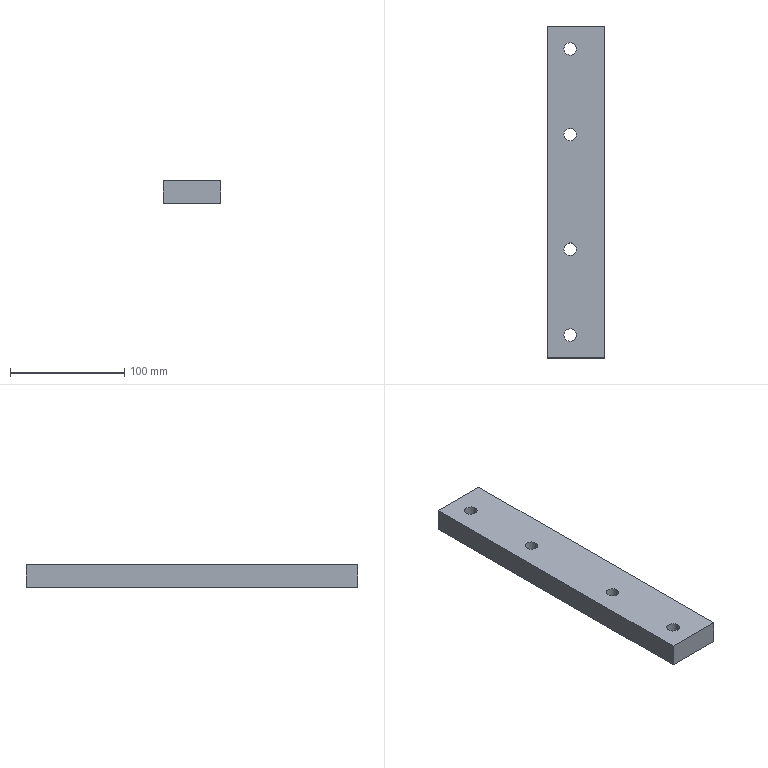Part | SolidWorks | features Extrusion 1, HoleWzd 1 | 1 solid | 14 faces | box 50 x 290 x 20 mm | volume 282397 mm3 | cylinder 8 | plane 6 | commonest cylinder face diameters 11 x8
STEP:
#1=CARTESIAN_POINT('',(0.5,125.,0.));
#2=VERTEX_POINT('',#1);
#3=CARTESIAN_POINT('',(-10.5,125.,0.));
#4=VERTEX_POINT('',#3);
#5=CARTESIAN_POINT('',(-5.,125.,0.));
#6=DIRECTION('',(0.,0.,-1.));
#7=DIRECTION('',(-1.,0.,0.));
#8=AXIS2_PLACEMENT_3D('',#5,#6,#7);
#9=CIRCLE('',#8,5.5);
#10=EDGE_CURVE('',#2,#4,#9,.T.);
#11=ORIENTED_EDGE('',*,*,#10,.T.);
#12=CARTESIAN_POINT('',(-10.5,125.,20.));
#13=VERTEX_POINT('',#12);
#14=CARTESIAN_POINT('',(-10.5,125.,20.));
#15=DIRECTION('',(0.,0.,1.));
#16=VECTOR('',#15,1000.);
#17=LINE('',#14,#16);
#18=EDGE_CURVE('',#4,#13,#17,.T.);
#19=ORIENTED_EDGE('',*,*,#18,.T.);
#20=CARTESIAN_POINT('',(0.5,125.,20.));
#21=VERTEX_POINT('',#20);
#22=CARTESIAN_POINT('',(-5.,125.,20.));
#23=DIRECTION('',(0.,0.,1.));
#24=DIRECTION('',(1.,0.,0.));
#25=AXIS2_PLACEMENT_3D('',#22,#23,#24);
#26=CIRCLE('',#25,5.5);
#27=EDGE_CURVE('',#13,#21,#26,.T.);
#28=ORIENTED_EDGE('',*,*,#27,.T.);
#29=CARTESIAN_POINT('',(0.5,125.,20.));
#30=DIRECTION('',(0.,0.,1.));
#31=VECTOR('',#30,1000.);
#32=LINE('',#29,#31);
#33=EDGE_CURVE('',#2,#21,#32,.T.);
#34=ORIENTED_EDGE('',*,*,#33,.F.);
#35=EDGE_LOOP('',(#11,#19,#28,#34));
#36=FACE_OUTER_BOUND('',#35,.T.);
#37=CARTESIAN_POINT('',(-5.,125.,20.));
#38=DIRECTION('',(0.,0.,1.));
#39=DIRECTION('',(1.,0.,0.));
#40=AXIS2_PLACEMENT_3D('',#37,#38,#39);
#41=CYLINDRICAL_SURFACE('',#40,5.5);
#42=ADVANCED_FACE('',(#36),#41,.F.);
#43=CARTESIAN_POINT('',(0.5,50.,0.));
#44=VERTEX_POINT('',#43);
#45=CARTESIAN_POINT('',(-10.5,50.,0.));
#46=VERTEX_POINT('',#45);
#47=CARTESIAN_POINT('',(-5.,50.,0.));
#48=DIRECTION('',(0.,0.,-1.));
#49=DIRECTION('',(-1.,0.,0.));
#50=AXIS2_PLACEMENT_3D('',#47,#48,#49);
#51=CIRCLE('',#50,5.5);
#52=EDGE_CURVE('',#44,#46,#51,.T.);
#53=ORIENTED_EDGE('',*,*,#52,.T.);
#54=CARTESIAN_POINT('',(-10.5,50.,20.));
#55=VERTEX_POINT('',#54);
#56=CARTESIAN_POINT('',(-10.5,50.,20.));
#57=DIRECTION('',(0.,0.,1.));
#58=VECTOR('',#57,1000.);
#59=LINE('',#56,#58);
#60=EDGE_CURVE('',#46,#55,#59,.T.);
#61=ORIENTED_EDGE('',*,*,#60,.T.);
#62=CARTESIAN_POINT('',(0.5,50.,20.));
#63=VERTEX_POINT('',#62);
#64=CARTESIAN_POINT('',(-5.,50.,20.));
#65=DIRECTION('',(0.,0.,1.));
#66=DIRECTION('',(1.,0.,0.));
#67=AXIS2_PLACEMENT_3D('',#64,#65,#66);
#68=CIRCLE('',#67,5.5);
#69=EDGE_CURVE('',#55,#63,#68,.T.);
#70=ORIENTED_EDGE('',*,*,#69,.T.);
#71=CARTESIAN_POINT('',(0.5,50.,20.));
#72=DIRECTION('',(0.,0.,1.));
#73=VECTOR('',#72,1000.);
#74=LINE('',#71,#73);
#75=EDGE_CURVE('',#44,#63,#74,.T.);
#76=ORIENTED_EDGE('',*,*,#75,.F.);
#77=EDGE_LOOP('',(#53,#61,#70,#76));
#78=FACE_OUTER_BOUND('',#77,.T.);
#79=CARTESIAN_POINT('',(-5.,50.,20.));
#80=DIRECTION('',(0.,0.,1.));
#81=DIRECTION('',(1.,0.,0.));
#82=AXIS2_PLACEMENT_3D('',#79,#80,#81);
#83=CYLINDRICAL_SURFACE('',#82,5.5);
#84=ADVANCED_FACE('',(#78),#83,.F.);
#85=CARTESIAN_POINT('',(0.5,-50.,0.));
#86=VERTEX_POINT('',#85);
#87=CARTESIAN_POINT('',(-10.5,-50.,0.));
#88=VERTEX_POINT('',#87);
#89=CARTESIAN_POINT('',(-5.,-50.,0.));
#90=DIRECTION('',(0.,0.,-1.));
#91=DIRECTION('',(-1.,0.,0.));
#92=AXIS2_PLACEMENT_3D('',#89,#90,#91);
#93=CIRCLE('',#92,5.5);
#94=EDGE_CURVE('',#86,#88,#93,.T.);
#95=ORIENTED_EDGE('',*,*,#94,.T.);
#96=CARTESIAN_POINT('',(-10.5,-50.,20.));
#97=VERTEX_POINT('',#96);
#98=CARTESIAN_POINT('',(-10.5,-50.,20.));
#99=DIRECTION('',(0.,0.,1.));
#100=VECTOR('',#99,1000.);
#101=LINE('',#98,#100);
#102=EDGE_CURVE('',#88,#97,#101,.T.);
#103=ORIENTED_EDGE('',*,*,#102,.T.);
#104=CARTESIAN_POINT('',(0.5,-50.,20.));
#105=VERTEX_POINT('',#104);
#106=CARTESIAN_POINT('',(-5.,-50.,20.));
#107=DIRECTION('',(0.,0.,1.));
#108=DIRECTION('',(1.,0.,0.));
#109=AXIS2_PLACEMENT_3D('',#106,#107,#108);
#110=CIRCLE('',#109,5.5);
#111=EDGE_CURVE('',#97,#105,#110,.T.);
#112=ORIENTED_EDGE('',*,*,#111,.T.);
#113=CARTESIAN_POINT('',(0.5,-50.,20.));
#114=DIRECTION('',(0.,0.,1.));
#115=VECTOR('',#114,1000.);
#116=LINE('',#113,#115);
#117=EDGE_CURVE('',#86,#105,#116,.T.);
#118=ORIENTED_EDGE('',*,*,#117,.F.);
#119=EDGE_LOOP('',(#95,#103,#112,#118));
#120=FACE_OUTER_BOUND('',#119,.T.);
#121=CARTESIAN_POINT('',(-5.,-50.,20.));
#122=DIRECTION('',(0.,0.,1.));
#123=DIRECTION('',(1.,0.,0.));
#124=AXIS2_PLACEMENT_3D('',#121,#122,#123);
#125=CYLINDRICAL_SURFACE('',#124,5.5);
#126=ADVANCED_FACE('',(#120),#125,.F.);
#127=CARTESIAN_POINT('',(0.5,-125.,0.));
#128=VERTEX_POINT('',#127);
#129=CARTESIAN_POINT('',(-10.5,-125.,0.));
#130=VERTEX_POINT('',#129);
#131=CARTESIAN_POINT('',(-5.,-125.,0.));
#132=DIRECTION('',(0.,0.,-1.));
#133=DIRECTION('',(-1.,0.,0.));
#134=AXIS2_PLACEMENT_3D('',#131,#132,#133);
#135=CIRCLE('',#134,5.5);
#136=EDGE_CURVE('',#128,#130,#135,.T.);
#137=ORIENTED_EDGE('',*,*,#136,.T.);
#138=CARTESIAN_POINT('',(-10.5,-125.,20.));
#139=VERTEX_POINT('',#138);
#140=CARTESIAN_POINT('',(-10.5,-125.,20.));
#141=DIRECTION('',(0.,0.,1.));
#142=VECTOR('',#141,1000.);
#143=LINE('',#140,#142);
#144=EDGE_CURVE('',#130,#139,#143,.T.);
#145=ORIENTED_EDGE('',*,*,#144,.T.);
#146=CARTESIAN_POINT('',(0.5,-125.,20.));
#147=VERTEX_POINT('',#146);
#148=CARTESIAN_POINT('',(-5.,-125.,20.));
#149=DIRECTION('',(0.,0.,1.));
#150=DIRECTION('',(1.,0.,0.));
#151=AXIS2_PLACEMENT_3D('',#148,#149,#150);
#152=CIRCLE('',#151,5.5);
#153=EDGE_CURVE('',#139,#147,#152,.T.);
#154=ORIENTED_EDGE('',*,*,#153,.T.);
#155=CARTESIAN_POINT('',(0.5,-125.,20.));
#156=DIRECTION('',(0.,0.,1.));
#157=VECTOR('',#156,1000.);
#158=LINE('',#155,#157);
#159=EDGE_CURVE('',#128,#147,#158,.T.);
#160=ORIENTED_EDGE('',*,*,#159,.F.);
#161=EDGE_LOOP('',(#137,#145,#154,#160));
#162=FACE_OUTER_BOUND('',#161,.T.);
#163=CARTESIAN_POINT('',(-5.,-125.,20.));
#164=DIRECTION('',(0.,0.,1.));
#165=DIRECTION('',(1.,0.,0.));
#166=AXIS2_PLACEMENT_3D('',#163,#164,#165);
#167=CYLINDRICAL_SURFACE('',#166,5.5);
#168=ADVANCED_FACE('',(#162),#167,.F.);
#169=CARTESIAN_POINT('',(25.,-145.,0.));
#170=VERTEX_POINT('',#169);
#171=CARTESIAN_POINT('',(25.,145.,0.));
#172=VERTEX_POINT('',#171);
#173=CARTESIAN_POINT('',(25.,-145.,0.));
#174=DIRECTION('',(0.,1.,0.));
#175=VECTOR('',#174,1000.);
#176=LINE('',#173,#175);
#177=EDGE_CURVE('',#170,#172,#176,.T.);
#178=ORIENTED_EDGE('',*,*,#177,.T.);
#179=CARTESIAN_POINT('',(25.,145.,20.));
#180=VERTEX_POINT('',#179);
#181=CARTESIAN_POINT('',(25.,145.,20.));
#182=DIRECTION('',(0.,0.,-1.));
#183=VECTOR('',#182,1000.);
#184=LINE('',#181,#183);
#185=EDGE_CURVE('',#180,#172,#184,.T.);
#186=ORIENTED_EDGE('',*,*,#185,.F.);
#187=CARTESIAN_POINT('',(25.,-145.,20.));
#188=VERTEX_POINT('',#187);
#189=CARTESIAN_POINT('',(25.,-145.,20.));
#190=DIRECTION('',(0.,1.,0.));
#191=VECTOR('',#190,1000.);
#192=LINE('',#189,#191);
#193=EDGE_CURVE('',#188,#180,#192,.T.);
#194=ORIENTED_EDGE('',*,*,#193,.F.);
#195=CARTESIAN_POINT('',(25.,-145.,20.));
#196=DIRECTION('',(0.,0.,-1.));
#197=VECTOR('',#196,1000.);
#198=LINE('',#195,#197);
#199=EDGE_CURVE('',#188,#170,#198,.T.);
#200=ORIENTED_EDGE('',*,*,#199,.T.);
#201=EDGE_LOOP('',(#178,#186,#194,#200));
#202=FACE_OUTER_BOUND('',#201,.T.);
#203=CARTESIAN_POINT('',(25.,-145.,20.));
#204=DIRECTION('',(-1.,0.,0.));
#205=DIRECTION('',(0.,0.,1.));
#206=AXIS2_PLACEMENT_3D('',#203,#204,#205);
#207=PLANE('',#206);
#208=ADVANCED_FACE('',(#202),#207,.F.);
#209=CARTESIAN_POINT('',(-25.,145.,0.));
#210=VERTEX_POINT('',#209);
#211=CARTESIAN_POINT('',(-25.,145.,0.));
#212=DIRECTION('',(-1.,0.,0.));
#213=VECTOR('',#212,1000.);
#214=LINE('',#211,#213);
#215=EDGE_CURVE('',#172,#210,#214,.T.);
#216=ORIENTED_EDGE('',*,*,#215,.T.);
#217=CARTESIAN_POINT('',(-25.,145.,20.));
#218=VERTEX_POINT('',#217);
#219=CARTESIAN_POINT('',(-25.,145.,20.));
#220=DIRECTION('',(0.,0.,-1.));
#221=VECTOR('',#220,1000.);
#222=LINE('',#219,#221);
#223=EDGE_CURVE('',#218,#210,#222,.T.);
#224=ORIENTED_EDGE('',*,*,#223,.F.);
#225=CARTESIAN_POINT('',(-25.,145.,20.));
#226=DIRECTION('',(-1.,0.,0.));
#227=VECTOR('',#226,1000.);
#228=LINE('',#225,#227);
#229=EDGE_CURVE('',#180,#218,#228,.T.);
#230=ORIENTED_EDGE('',*,*,#229,.F.);
#231=ORIENTED_EDGE('',*,*,#185,.T.);
#232=EDGE_LOOP('',(#216,#224,#230,#231));
#233=FACE_OUTER_BOUND('',#232,.T.);
#234=CARTESIAN_POINT('',(-25.,145.,20.));
#235=DIRECTION('',(0.,-1.,0.));
#236=DIRECTION('',(0.,0.,-1.));
#237=AXIS2_PLACEMENT_3D('',#234,#235,#236);
#238=PLANE('',#237);
#239=ADVANCED_FACE('',(#233),#238,.F.);
#240=CARTESIAN_POINT('',(-25.,-145.,0.));
#241=VERTEX_POINT('',#240);
#242=CARTESIAN_POINT('',(-25.,-145.,0.));
#243=DIRECTION('',(0.,-1.,0.));
#244=VECTOR('',#243,1000.);
#245=LINE('',#242,#244);
#246=EDGE_CURVE('',#210,#241,#245,.T.);
#247=ORIENTED_EDGE('',*,*,#246,.T.);
#248=CARTESIAN_POINT('',(-25.,-145.,20.));
#249=VERTEX_POINT('',#248);
#250=CARTESIAN_POINT('',(-25.,-145.,20.));
#251=DIRECTION('',(0.,0.,-1.));
#252=VECTOR('',#251,1000.);
#253=LINE('',#250,#252);
#254=EDGE_CURVE('',#249,#241,#253,.T.);
#255=ORIENTED_EDGE('',*,*,#254,.F.);
#256=CARTESIAN_POINT('',(-25.,-145.,20.));
#257=DIRECTION('',(0.,-1.,0.));
#258=VECTOR('',#257,1000.);
#259=LINE('',#256,#258);
#260=EDGE_CURVE('',#218,#249,#259,.T.);
#261=ORIENTED_EDGE('',*,*,#260,.F.);
#262=ORIENTED_EDGE('',*,*,#223,.T.);
#263=EDGE_LOOP('',(#247,#255,#261,#262));
#264=FACE_OUTER_BOUND('',#263,.T.);
#265=CARTESIAN_POINT('',(-25.,-145.,20.));
#266=DIRECTION('',(1.,0.,0.));
#267=DIRECTION('',(0.,0.,-1.));
#268=AXIS2_PLACEMENT_3D('',#265,#266,#267);
#269=PLANE('',#268);
#270=ADVANCED_FACE('',(#264),#269,.F.);
#271=CARTESIAN_POINT('',(-25.,-145.,0.));
#272=DIRECTION('',(1.,0.,0.));
#273=VECTOR('',#272,1000.);
#274=LINE('',#271,#273);
#275=EDGE_CURVE('',#241,#170,#274,.T.);
#276=ORIENTED_EDGE('',*,*,#275,.T.);
#277=ORIENTED_EDGE('',*,*,#199,.F.);
#278=CARTESIAN_POINT('',(-25.,-145.,20.));
#279=DIRECTION('',(1.,0.,0.));
#280=VECTOR('',#279,1000.);
#281=LINE('',#278,#280);
#282=EDGE_CURVE('',#249,#188,#281,.T.);
#283=ORIENTED_EDGE('',*,*,#282,.F.);
#284=ORIENTED_EDGE('',*,*,#254,.T.);
#285=EDGE_LOOP('',(#276,#277,#283,#284));
#286=FACE_OUTER_BOUND('',#285,.T.);
#287=CARTESIAN_POINT('',(-25.,-145.,20.));
#288=DIRECTION('',(0.,1.,0.));
#289=DIRECTION('',(0.,0.,1.));
#290=AXIS2_PLACEMENT_3D('',#287,#288,#289);
#291=PLANE('',#290);
#292=ADVANCED_FACE('',(#286),#291,.F.);
#293=CARTESIAN_POINT('',(-5.,125.,20.));
#294=DIRECTION('',(0.,0.,1.));
#295=DIRECTION('',(1.,0.,0.));
#296=AXIS2_PLACEMENT_3D('',#293,#294,#295);
#297=CIRCLE('',#296,5.5);
#298=EDGE_CURVE('',#21,#13,#297,.T.);
#299=ORIENTED_EDGE('',*,*,#298,.F.);
#300=ORIENTED_EDGE('',*,*,#27,.F.);
#301=EDGE_LOOP('',(#299,#300));
#302=FACE_BOUND('',#301,.T.);
#303=CARTESIAN_POINT('',(-5.,50.,20.));
#304=DIRECTION('',(0.,0.,1.));
#305=DIRECTION('',(1.,0.,0.));
#306=AXIS2_PLACEMENT_3D('',#303,#304,#305);
#307=CIRCLE('',#306,5.5);
#308=EDGE_CURVE('',#63,#55,#307,.T.);
#309=ORIENTED_EDGE('',*,*,#308,.F.);
#310=ORIENTED_EDGE('',*,*,#69,.F.);
#311=EDGE_LOOP('',(#309,#310));
#312=FACE_BOUND('',#311,.T.);
#313=CARTESIAN_POINT('',(-5.,-50.,20.));
#314=DIRECTION('',(0.,0.,1.));
#315=DIRECTION('',(1.,0.,0.));
#316=AXIS2_PLACEMENT_3D('',#313,#314,#315);
#317=CIRCLE('',#316,5.5);
#318=EDGE_CURVE('',#105,#97,#317,.T.);
#319=ORIENTED_EDGE('',*,*,#318,.F.);
#320=ORIENTED_EDGE('',*,*,#111,.F.);
#321=EDGE_LOOP('',(#319,#320));
#322=FACE_BOUND('',#321,.T.);
#323=CARTESIAN_POINT('',(-5.,-125.,20.));
#324=DIRECTION('',(0.,0.,1.));
#325=DIRECTION('',(1.,0.,0.));
#326=AXIS2_PLACEMENT_3D('',#323,#324,#325);
#327=CIRCLE('',#326,5.5);
#328=EDGE_CURVE('',#147,#139,#327,.T.);
#329=ORIENTED_EDGE('',*,*,#328,.F.);
#330=ORIENTED_EDGE('',*,*,#153,.F.);
#331=EDGE_LOOP('',(#329,#330));
#332=FACE_BOUND('',#331,.T.);
#333=ORIENTED_EDGE('',*,*,#193,.T.);
#334=ORIENTED_EDGE('',*,*,#229,.T.);
#335=ORIENTED_EDGE('',*,*,#260,.T.);
#336=ORIENTED_EDGE('',*,*,#282,.T.);
#337=EDGE_LOOP('',(#333,#334,#335,#336));
#338=FACE_OUTER_BOUND('',#337,.T.);
#339=CARTESIAN_POINT('',(0.,0.,20.));
#340=DIRECTION('',(0.,0.,-1.));
#341=DIRECTION('',(-1.,0.,0.));
#342=AXIS2_PLACEMENT_3D('',#339,#340,#341);
#343=PLANE('',#342);
#344=ADVANCED_FACE('',(#302,#312,#322,#332,#338),#343,.F.);
#345=ORIENTED_EDGE('',*,*,#10,.F.);
#346=CARTESIAN_POINT('',(-5.,125.,0.));
#347=DIRECTION('',(0.,0.,-1.));
#348=DIRECTION('',(-1.,0.,0.));
#349=AXIS2_PLACEMENT_3D('',#346,#347,#348);
#350=CIRCLE('',#349,5.5);
#351=EDGE_CURVE('',#4,#2,#350,.T.);
#352=ORIENTED_EDGE('',*,*,#351,.F.);
#353=EDGE_LOOP('',(#345,#352));
#354=FACE_BOUND('',#353,.T.);
#355=ORIENTED_EDGE('',*,*,#52,.F.);
#356=CARTESIAN_POINT('',(-5.,50.,0.));
#357=DIRECTION('',(0.,0.,-1.));
#358=DIRECTION('',(-1.,0.,0.));
#359=AXIS2_PLACEMENT_3D('',#356,#357,#358);
#360=CIRCLE('',#359,5.5);
#361=EDGE_CURVE('',#46,#44,#360,.T.);
#362=ORIENTED_EDGE('',*,*,#361,.F.);
#363=EDGE_LOOP('',(#355,#362));
#364=FACE_BOUND('',#363,.T.);
#365=ORIENTED_EDGE('',*,*,#94,.F.);
#366=CARTESIAN_POINT('',(-5.,-50.,0.));
#367=DIRECTION('',(0.,0.,-1.));
#368=DIRECTION('',(-1.,0.,0.));
#369=AXIS2_PLACEMENT_3D('',#366,#367,#368);
#370=CIRCLE('',#369,5.5);
#371=EDGE_CURVE('',#88,#86,#370,.T.);
#372=ORIENTED_EDGE('',*,*,#371,.F.);
#373=EDGE_LOOP('',(#365,#372));
#374=FACE_BOUND('',#373,.T.);
#375=ORIENTED_EDGE('',*,*,#136,.F.);
#376=CARTESIAN_POINT('',(-5.,-125.,0.));
#377=DIRECTION('',(0.,0.,-1.));
#378=DIRECTION('',(-1.,0.,0.));
#379=AXIS2_PLACEMENT_3D('',#376,#377,#378);
#380=CIRCLE('',#379,5.5);
#381=EDGE_CURVE('',#130,#128,#380,.T.);
#382=ORIENTED_EDGE('',*,*,#381,.F.);
#383=EDGE_LOOP('',(#375,#382));
#384=FACE_BOUND('',#383,.T.);
#385=ORIENTED_EDGE('',*,*,#177,.F.);
#386=ORIENTED_EDGE('',*,*,#275,.F.);
#387=ORIENTED_EDGE('',*,*,#246,.F.);
#388=ORIENTED_EDGE('',*,*,#215,.F.);
#389=EDGE_LOOP('',(#385,#386,#387,#388));
#390=FACE_OUTER_BOUND('',#389,.T.);
#391=CARTESIAN_POINT('',(0.,0.,0.));
#392=DIRECTION('',(0.,0.,-1.));
#393=DIRECTION('',(-1.,0.,0.));
#394=AXIS2_PLACEMENT_3D('',#391,#392,#393);
#395=PLANE('',#394);
#396=ADVANCED_FACE('',(#354,#364,#374,#384,#390),#395,.T.);
#397=ORIENTED_EDGE('',*,*,#144,.F.);
#398=ORIENTED_EDGE('',*,*,#381,.T.);
#399=ORIENTED_EDGE('',*,*,#159,.T.);
#400=ORIENTED_EDGE('',*,*,#328,.T.);
#401=EDGE_LOOP('',(#397,#398,#399,#400));
#402=FACE_OUTER_BOUND('',#401,.T.);
#403=CARTESIAN_POINT('',(-5.,-125.,20.));
#404=DIRECTION('',(0.,0.,1.));
#405=DIRECTION('',(1.,0.,0.));
#406=AXIS2_PLACEMENT_3D('',#403,#404,#405);
#407=CYLINDRICAL_SURFACE('',#406,5.5);
#408=ADVANCED_FACE('',(#402),#407,.F.);
#409=ORIENTED_EDGE('',*,*,#102,.F.);
#410=ORIENTED_EDGE('',*,*,#371,.T.);
#411=ORIENTED_EDGE('',*,*,#117,.T.);
#412=ORIENTED_EDGE('',*,*,#318,.T.);
#413=EDGE_LOOP('',(#409,#410,#411,#412));
#414=FACE_OUTER_BOUND('',#413,.T.);
#415=CARTESIAN_POINT('',(-5.,-50.,20.));
#416=DIRECTION('',(0.,0.,1.));
#417=DIRECTION('',(1.,0.,0.));
#418=AXIS2_PLACEMENT_3D('',#415,#416,#417);
#419=CYLINDRICAL_SURFACE('',#418,5.5);
#420=ADVANCED_FACE('',(#414),#419,.F.);
#421=ORIENTED_EDGE('',*,*,#60,.F.);
#422=ORIENTED_EDGE('',*,*,#361,.T.);
#423=ORIENTED_EDGE('',*,*,#75,.T.);
#424=ORIENTED_EDGE('',*,*,#308,.T.);
#425=EDGE_LOOP('',(#421,#422,#423,#424));
#426=FACE_OUTER_BOUND('',#425,.T.);
#427=CARTESIAN_POINT('',(-5.,50.,20.));
#428=DIRECTION('',(0.,0.,1.));
#429=DIRECTION('',(1.,0.,0.));
#430=AXIS2_PLACEMENT_3D('',#427,#428,#429);
#431=CYLINDRICAL_SURFACE('',#430,5.5);
#432=ADVANCED_FACE('',(#426),#431,.F.);
#433=ORIENTED_EDGE('',*,*,#18,.F.);
#434=ORIENTED_EDGE('',*,*,#351,.T.);
#435=ORIENTED_EDGE('',*,*,#33,.T.);
#436=ORIENTED_EDGE('',*,*,#298,.T.);
#437=EDGE_LOOP('',(#433,#434,#435,#436));
#438=FACE_OUTER_BOUND('',#437,.T.);
#439=CARTESIAN_POINT('',(-5.,125.,20.));
#440=DIRECTION('',(0.,0.,1.));
#441=DIRECTION('',(1.,0.,0.));
#442=AXIS2_PLACEMENT_3D('',#439,#440,#441);
#443=CYLINDRICAL_SURFACE('',#442,5.5);
#444=ADVANCED_FACE('',(#438),#443,.F.);
#445=CLOSED_SHELL('',(#42,#84,#126,#168,#208,#239,#270,#292,#344,#396,#408,#420,#432,#444));
#446=MANIFOLD_SOLID_BREP('',#445);
#447=CARTESIAN_POINT('',(0.,0.,0.));
#448=DIRECTION('',(0.,0.,1.));
#449=DIRECTION('',(1.,0.,0.));
#450=AXIS2_PLACEMENT_3D('',#447,#448,#449);
#451=(LENGTH_UNIT()NAMED_UNIT(*)SI_UNIT(.MILLI.,.METRE.));
#452=UNCERTAINTY_MEASURE_WITH_UNIT(LENGTH_MEASURE(0.00001),#451,'','');
#453=(NAMED_UNIT(*)PLANE_ANGLE_UNIT()SI_UNIT($,.RADIAN.));
#454=(NAMED_UNIT(*)SI_UNIT($,.STERADIAN.)SOLID_ANGLE_UNIT());
#455=(GEOMETRIC_REPRESENTATION_CONTEXT(3)GLOBAL_UNCERTAINTY_ASSIGNED_CONTEXT((#452))GLOBAL_UNIT_ASSIGNED_CONTEXT((#451,#453,#454))REPRESENTATION_CONTEXT('',''));
#456=ADVANCED_BREP_SHAPE_REPRESENTATION('',(#446,#450),#455);